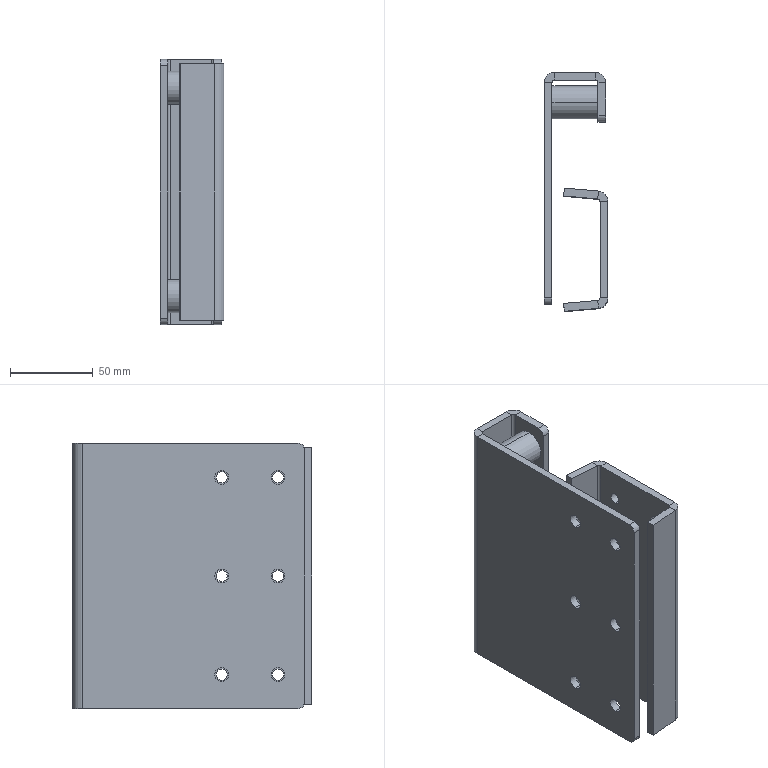Part | STEP file | BASE RODILLOS FRONTALES | 4 solids | 98 faces | box 38.52 x 144.159 x 160 mm | volume 238623 mm3 | cylinder 52 | plane 42 | cone 4 | commonest cylinder face diameters 6.8 x12 8.4 x12 16 x8 3 x4 8 x4 8.5 x4